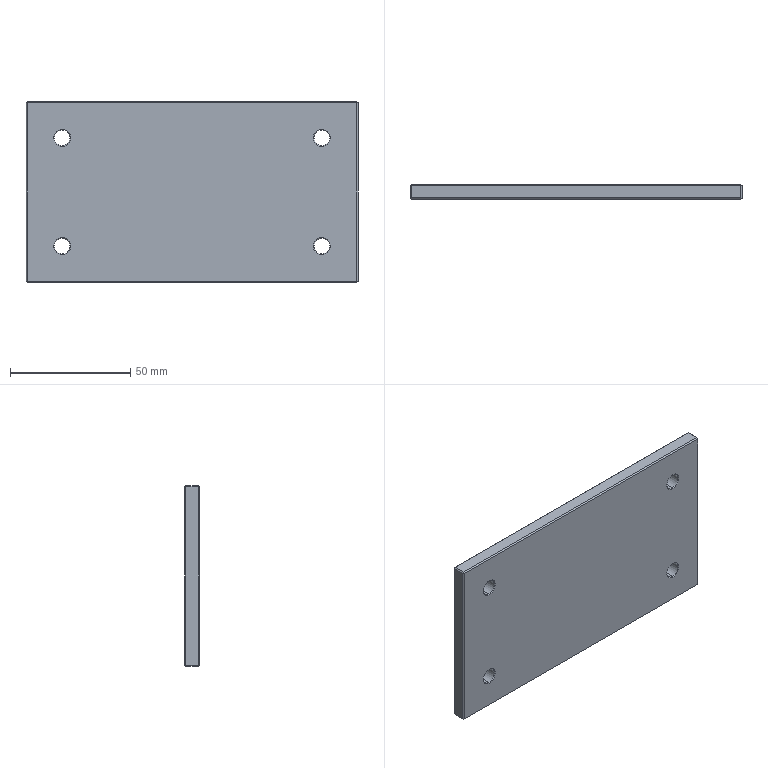Part | STEP file | 10040 | 1 solid | 42 faces | box 138 x 6 x 75 mm | volume 61187 mm3 | plane 18 | cone 16 | cylinder 8 | commonest cylinder face diameters 6.5 x8